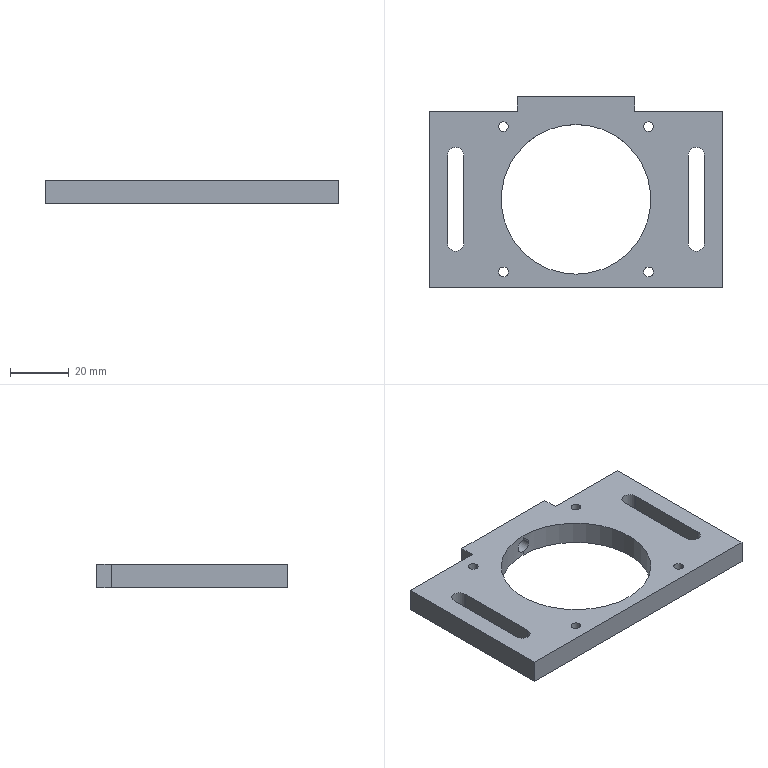Part | NX | features BREP 1 | 1 solid | 30 faces | box 100.003 x 65.003 x 8 mm | volume 29776 mm3 | cylinder 16 | plane 14 | commonest cylinder face diameters 3.3 x8 5.5 x4 5 x2 51 x2
STEP:
#1=CARTESIAN_POINT('',(-574.028,37.759,0.));
#2=VERTEX_POINT('',#1);
#3=CARTESIAN_POINT('',(-570.728,37.759,0.));
#4=VERTEX_POINT('',#3);
#5=CARTESIAN_POINT('',(-572.378,37.759,0.));
#6=DIRECTION('',(0.,0.,1.));
#7=DIRECTION('',(1.,0.,0.));
#8=AXIS2_PLACEMENT_3D('',#5,#6,#7);
#9=CIRCLE('',#8,1.65);
#10=EDGE_CURVE('',#2,#4,#9,.T.);
#11=ORIENTED_EDGE('',*,*,#10,.F.);
#12=CARTESIAN_POINT('',(-574.028,37.759,8.));
#13=VERTEX_POINT('',#12);
#14=CARTESIAN_POINT('',(-574.028,37.759,8.));
#15=DIRECTION('',(0.,0.,1.));
#16=VECTOR('',#15,1000.);
#17=LINE('',#14,#16);
#18=EDGE_CURVE('',#13,#2,#17,.F.);
#19=ORIENTED_EDGE('',*,*,#18,.F.);
#20=CARTESIAN_POINT('',(-570.728,37.759,8.));
#21=VERTEX_POINT('',#20);
#22=CARTESIAN_POINT('',(-572.378,37.759,8.));
#23=DIRECTION('',(0.,0.,1.));
#24=DIRECTION('',(1.,0.,0.));
#25=AXIS2_PLACEMENT_3D('',#22,#23,#24);
#26=CIRCLE('',#25,1.65);
#27=EDGE_CURVE('',#13,#21,#26,.T.);
#28=ORIENTED_EDGE('',*,*,#27,.T.);
#29=CARTESIAN_POINT('',(-570.728,37.759,8.));
#30=DIRECTION('',(0.,0.,1.));
#31=VECTOR('',#30,1000.);
#32=LINE('',#29,#31);
#33=EDGE_CURVE('',#21,#4,#32,.F.);
#34=ORIENTED_EDGE('',*,*,#33,.T.);
#35=EDGE_LOOP('',(#11,#19,#28,#34));
#36=FACE_BOUND('',#35,.T.);
#37=CARTESIAN_POINT('',(-572.378,37.759,8.));
#38=DIRECTION('',(0.,0.,1.));
#39=DIRECTION('',(1.,0.,0.));
#40=AXIS2_PLACEMENT_3D('',#37,#38,#39);
#41=CYLINDRICAL_SURFACE('',#40,1.65);
#42=ADVANCED_FACE('',(#36),#41,.F.);
#43=CARTESIAN_POINT('',(-524.531,37.761,0.));
#44=VERTEX_POINT('',#43);
#45=CARTESIAN_POINT('',(-521.231,37.761,0.));
#46=VERTEX_POINT('',#45);
#47=CARTESIAN_POINT('',(-522.881,37.761,0.));
#48=DIRECTION('',(0.,0.,1.));
#49=DIRECTION('',(1.,0.,0.));
#50=AXIS2_PLACEMENT_3D('',#47,#48,#49);
#51=CIRCLE('',#50,1.65);
#52=EDGE_CURVE('',#44,#46,#51,.T.);
#53=ORIENTED_EDGE('',*,*,#52,.F.);
#54=CARTESIAN_POINT('',(-524.531,37.761,8.));
#55=VERTEX_POINT('',#54);
#56=CARTESIAN_POINT('',(-524.531,37.761,8.));
#57=DIRECTION('',(0.,0.,1.));
#58=VECTOR('',#57,1000.);
#59=LINE('',#56,#58);
#60=EDGE_CURVE('',#55,#44,#59,.F.);
#61=ORIENTED_EDGE('',*,*,#60,.F.);
#62=CARTESIAN_POINT('',(-521.231,37.761,8.));
#63=VERTEX_POINT('',#62);
#64=CARTESIAN_POINT('',(-522.881,37.761,8.));
#65=DIRECTION('',(0.,0.,1.));
#66=DIRECTION('',(1.,0.,0.));
#67=AXIS2_PLACEMENT_3D('',#64,#65,#66);
#68=CIRCLE('',#67,1.65);
#69=EDGE_CURVE('',#55,#63,#68,.T.);
#70=ORIENTED_EDGE('',*,*,#69,.T.);
#71=CARTESIAN_POINT('',(-521.231,37.761,8.));
#72=DIRECTION('',(0.,0.,1.));
#73=VECTOR('',#72,1000.);
#74=LINE('',#71,#73);
#75=EDGE_CURVE('',#63,#46,#74,.F.);
#76=ORIENTED_EDGE('',*,*,#75,.T.);
#77=EDGE_LOOP('',(#53,#61,#70,#76));
#78=FACE_BOUND('',#77,.T.);
#79=CARTESIAN_POINT('',(-522.881,37.761,8.));
#80=DIRECTION('',(0.,0.,1.));
#81=DIRECTION('',(1.,0.,0.));
#82=AXIS2_PLACEMENT_3D('',#79,#80,#81);
#83=CYLINDRICAL_SURFACE('',#82,1.65);
#84=ADVANCED_FACE('',(#78),#83,.F.);
#85=CARTESIAN_POINT('',(-524.529,-11.736,0.));
#86=VERTEX_POINT('',#85);
#87=CARTESIAN_POINT('',(-521.229,-11.736,0.));
#88=VERTEX_POINT('',#87);
#89=CARTESIAN_POINT('',(-522.879,-11.736,0.));
#90=DIRECTION('',(0.,0.,1.));
#91=DIRECTION('',(1.,0.,0.));
#92=AXIS2_PLACEMENT_3D('',#89,#90,#91);
#93=CIRCLE('',#92,1.65);
#94=EDGE_CURVE('',#86,#88,#93,.T.);
#95=ORIENTED_EDGE('',*,*,#94,.F.);
#96=CARTESIAN_POINT('',(-524.529,-11.736,8.));
#97=VERTEX_POINT('',#96);
#98=CARTESIAN_POINT('',(-524.529,-11.736,8.));
#99=DIRECTION('',(0.,0.,1.));
#100=VECTOR('',#99,1000.);
#101=LINE('',#98,#100);
#102=EDGE_CURVE('',#97,#86,#101,.F.);
#103=ORIENTED_EDGE('',*,*,#102,.F.);
#104=CARTESIAN_POINT('',(-521.229,-11.736,8.));
#105=VERTEX_POINT('',#104);
#106=CARTESIAN_POINT('',(-522.879,-11.736,8.));
#107=DIRECTION('',(0.,0.,1.));
#108=DIRECTION('',(1.,0.,0.));
#109=AXIS2_PLACEMENT_3D('',#106,#107,#108);
#110=CIRCLE('',#109,1.65);
#111=EDGE_CURVE('',#97,#105,#110,.T.);
#112=ORIENTED_EDGE('',*,*,#111,.T.);
#113=CARTESIAN_POINT('',(-521.229,-11.736,8.));
#114=DIRECTION('',(0.,0.,1.));
#115=VECTOR('',#114,1000.);
#116=LINE('',#113,#115);
#117=EDGE_CURVE('',#105,#88,#116,.F.);
#118=ORIENTED_EDGE('',*,*,#117,.T.);
#119=EDGE_LOOP('',(#95,#103,#112,#118));
#120=FACE_BOUND('',#119,.T.);
#121=CARTESIAN_POINT('',(-522.879,-11.736,8.));
#122=DIRECTION('',(0.,0.,1.));
#123=DIRECTION('',(1.,0.,0.));
#124=AXIS2_PLACEMENT_3D('',#121,#122,#123);
#125=CYLINDRICAL_SURFACE('',#124,1.65);
#126=ADVANCED_FACE('',(#120),#125,.F.);
#127=CARTESIAN_POINT('',(-574.026,-11.739,0.));
#128=VERTEX_POINT('',#127);
#129=CARTESIAN_POINT('',(-570.726,-11.739,0.));
#130=VERTEX_POINT('',#129);
#131=CARTESIAN_POINT('',(-572.376,-11.739,0.));
#132=DIRECTION('',(0.,0.,1.));
#133=DIRECTION('',(1.,0.,0.));
#134=AXIS2_PLACEMENT_3D('',#131,#132,#133);
#135=CIRCLE('',#134,1.65);
#136=EDGE_CURVE('',#128,#130,#135,.T.);
#137=ORIENTED_EDGE('',*,*,#136,.F.);
#138=CARTESIAN_POINT('',(-574.026,-11.739,8.));
#139=VERTEX_POINT('',#138);
#140=CARTESIAN_POINT('',(-574.026,-11.739,8.));
#141=DIRECTION('',(0.,0.,1.));
#142=VECTOR('',#141,1000.);
#143=LINE('',#140,#142);
#144=EDGE_CURVE('',#139,#128,#143,.F.);
#145=ORIENTED_EDGE('',*,*,#144,.F.);
#146=CARTESIAN_POINT('',(-570.726,-11.739,8.));
#147=VERTEX_POINT('',#146);
#148=CARTESIAN_POINT('',(-572.376,-11.739,8.));
#149=DIRECTION('',(0.,0.,1.));
#150=DIRECTION('',(1.,0.,0.));
#151=AXIS2_PLACEMENT_3D('',#148,#149,#150);
#152=CIRCLE('',#151,1.65);
#153=EDGE_CURVE('',#139,#147,#152,.T.);
#154=ORIENTED_EDGE('',*,*,#153,.T.);
#155=CARTESIAN_POINT('',(-570.726,-11.739,8.));
#156=DIRECTION('',(0.,0.,1.));
#157=VECTOR('',#156,1000.);
#158=LINE('',#155,#157);
#159=EDGE_CURVE('',#147,#130,#158,.F.);
#160=ORIENTED_EDGE('',*,*,#159,.T.);
#161=EDGE_LOOP('',(#137,#145,#154,#160));
#162=FACE_BOUND('',#161,.T.);
#163=CARTESIAN_POINT('',(-572.376,-11.739,8.));
#164=DIRECTION('',(0.,0.,1.));
#165=DIRECTION('',(1.,0.,0.));
#166=AXIS2_PLACEMENT_3D('',#163,#164,#165);
#167=CYLINDRICAL_SURFACE('',#166,1.65);
#168=ADVANCED_FACE('',(#162),#167,.F.);
#169=CARTESIAN_POINT('',(-545.13,38.389,4.));
#170=VERTEX_POINT('',#169);
#171=CARTESIAN_POINT('',(-547.628,38.511,1.5));
#172=VERTEX_POINT('',#171);
#173=CARTESIAN_POINT('',(-547.628,38.511,1.5));
#174=CARTESIAN_POINT('',(-547.474,38.511,1.5));
#175=CARTESIAN_POINT('',(-547.166,38.509,1.523));
#176=CARTESIAN_POINT('',(-546.63,38.493,1.695));
#177=CARTESIAN_POINT('',(-546.34,38.479,1.843));
#178=CARTESIAN_POINT('',(-545.839,38.45,2.211));
#179=CARTESIAN_POINT('',(-545.471,38.421,2.714));
#180=CARTESIAN_POINT('',(-545.324,38.407,3.002));
#181=CARTESIAN_POINT('',(-545.152,38.391,3.538));
#182=CARTESIAN_POINT('',(-545.13,38.389,3.845));
#183=CARTESIAN_POINT('',(-545.13,38.389,4.));
#184=B_SPLINE_CURVE_WITH_KNOTS('',3,(#173,#174,#175,#176,#177,#178,#179,#180,#181,#182,#183),.UNSPECIFIED.,.F.,.F.,(4,1,1,1,1,1,1,1,4),(0.,0.125,0.25,0.375,0.5,0.625,0.75,0.875,1.),.UNSPECIFIED.);
#185=EDGE_CURVE('',#170,#172,#184,.F.);
#186=ORIENTED_EDGE('',*,*,#185,.F.);
#187=CARTESIAN_POINT('',(-545.13,48.011,4.));
#188=VERTEX_POINT('',#187);
#189=CARTESIAN_POINT('',(-545.13,48.011,4.));
#190=DIRECTION('',(-0.0000463,1.,0.));
#191=VECTOR('',#190,1000.);
#192=LINE('',#189,#191);
#193=EDGE_CURVE('',#170,#188,#192,.T.);
#194=ORIENTED_EDGE('',*,*,#193,.T.);
#195=CARTESIAN_POINT('',(-550.13,48.011,4.));
#196=VERTEX_POINT('',#195);
#197=CARTESIAN_POINT('',(-547.63,48.011,4.));
#198=DIRECTION('',(-0.0000463,1.,0.));
#199=DIRECTION('',(-1.,-0.0000463,0.));
#200=AXIS2_PLACEMENT_3D('',#197,#198,#199);
#201=CIRCLE('',#200,2.5);
#202=EDGE_CURVE('',#188,#196,#201,.T.);
#203=ORIENTED_EDGE('',*,*,#202,.T.);
#204=CARTESIAN_POINT('',(-550.13,38.388,4.));
#205=VERTEX_POINT('',#204);
#206=CARTESIAN_POINT('',(-550.13,48.011,4.));
#207=DIRECTION('',(-0.0000463,1.,0.));
#208=VECTOR('',#207,1000.);
#209=LINE('',#206,#208);
#210=EDGE_CURVE('',#205,#196,#209,.T.);
#211=ORIENTED_EDGE('',*,*,#210,.F.);
#212=CARTESIAN_POINT('',(-550.13,38.388,4.));
#213=CARTESIAN_POINT('',(-550.13,38.388,3.845));
#214=CARTESIAN_POINT('',(-550.107,38.391,3.537));
#215=CARTESIAN_POINT('',(-549.934,38.407,2.999));
#216=CARTESIAN_POINT('',(-549.787,38.42,2.712));
#217=CARTESIAN_POINT('',(-549.418,38.45,2.208));
#218=CARTESIAN_POINT('',(-548.918,38.479,1.843));
#219=CARTESIAN_POINT('',(-548.627,38.493,1.694));
#220=CARTESIAN_POINT('',(-548.091,38.509,1.522));
#221=CARTESIAN_POINT('',(-547.783,38.511,1.5));
#222=CARTESIAN_POINT('',(-547.628,38.511,1.5));
#223=B_SPLINE_CURVE_WITH_KNOTS('',3,(#212,#213,#214,#215,#216,#217,#218,#219,#220,#221,#222),.UNSPECIFIED.,.F.,.F.,(4,1,1,1,1,1,1,1,4),(0.,0.125,0.25,0.375,0.5,0.625,0.75,0.875,1.),.UNSPECIFIED.);
#224=EDGE_CURVE('',#172,#205,#223,.F.);
#225=ORIENTED_EDGE('',*,*,#224,.F.);
#226=EDGE_LOOP('',(#186,#194,#203,#211,#225));
#227=FACE_BOUND('',#226,.T.);
#228=CARTESIAN_POINT('',(-547.63,48.011,4.));
#229=DIRECTION('',(-0.0000463,1.,0.));
#230=DIRECTION('',(-1.,-0.0000463,0.));
#231=AXIS2_PLACEMENT_3D('',#228,#229,#230);
#232=CYLINDRICAL_SURFACE('',#231,2.5);
#233=ADVANCED_FACE('',(#227),#232,.F.);
#234=CARTESIAN_POINT('',(-547.628,38.511,0.));
#235=VERTEX_POINT('',#234);
#236=CARTESIAN_POINT('',(-547.628,-12.489,0.));
#237=VERTEX_POINT('',#236);
#238=CARTESIAN_POINT('',(-547.628,13.011,0.));
#239=DIRECTION('',(0.,0.,1.));
#240=DIRECTION('',(0.,-1.,0.));
#241=AXIS2_PLACEMENT_3D('',#238,#239,#240);
#242=CIRCLE('',#241,25.5);
#243=EDGE_CURVE('',#235,#237,#242,.T.);
#244=ORIENTED_EDGE('',*,*,#243,.F.);
#245=CARTESIAN_POINT('',(-547.628,38.511,0.));
#246=DIRECTION('',(0.,0.,1.));
#247=VECTOR('',#246,1000.);
#248=LINE('',#245,#247);
#249=EDGE_CURVE('',#172,#235,#248,.F.);
#250=ORIENTED_EDGE('',*,*,#249,.F.);
#251=ORIENTED_EDGE('',*,*,#224,.T.);
#252=CARTESIAN_POINT('',(-547.628,38.511,6.5));
#253=VERTEX_POINT('',#252);
#254=CARTESIAN_POINT('',(-550.13,38.388,4.));
#255=CARTESIAN_POINT('',(-550.13,38.388,4.657));
#256=CARTESIAN_POINT('',(-549.585,38.45,5.959));
#257=CARTESIAN_POINT('',(-548.285,38.511,6.5));
#258=CARTESIAN_POINT('',(-547.628,38.511,6.5));
#259=B_SPLINE_CURVE_WITH_KNOTS('',3,(#254,#255,#256,#257,#258),.UNSPECIFIED.,.F.,.F.,(4,1,4),(0.,0.5,1.),.UNSPECIFIED.);
#260=EDGE_CURVE('',#205,#253,#259,.T.);
#261=ORIENTED_EDGE('',*,*,#260,.T.);
#262=CARTESIAN_POINT('',(-547.628,38.511,8.));
#263=VERTEX_POINT('',#262);
#264=CARTESIAN_POINT('',(-547.628,38.511,0.));
#265=DIRECTION('',(0.,0.,1.));
#266=VECTOR('',#265,1000.);
#267=LINE('',#264,#266);
#268=EDGE_CURVE('',#253,#263,#267,.T.);
#269=ORIENTED_EDGE('',*,*,#268,.T.);
#270=CARTESIAN_POINT('',(-547.628,-12.489,8.));
#271=VERTEX_POINT('',#270);
#272=CARTESIAN_POINT('',(-547.628,13.011,8.));
#273=DIRECTION('',(0.,0.,1.));
#274=DIRECTION('',(0.,-1.,0.));
#275=AXIS2_PLACEMENT_3D('',#272,#273,#274);
#276=CIRCLE('',#275,25.5);
#277=EDGE_CURVE('',#263,#271,#276,.T.);
#278=ORIENTED_EDGE('',*,*,#277,.T.);
#279=CARTESIAN_POINT('',(-547.628,-12.489,0.));
#280=DIRECTION('',(0.,0.,1.));
#281=VECTOR('',#280,1000.);
#282=LINE('',#279,#281);
#283=EDGE_CURVE('',#271,#237,#282,.F.);
#284=ORIENTED_EDGE('',*,*,#283,.T.);
#285=EDGE_LOOP('',(#244,#250,#251,#261,#269,#278,#284));
#286=FACE_BOUND('',#285,.T.);
#287=CARTESIAN_POINT('',(-547.628,13.011,0.));
#288=DIRECTION('',(0.,0.,1.));
#289=DIRECTION('',(0.,-1.,0.));
#290=AXIS2_PLACEMENT_3D('',#287,#288,#289);
#291=CYLINDRICAL_SURFACE('',#290,25.5);
#292=ADVANCED_FACE('',(#286),#291,.F.);
#293=CARTESIAN_POINT('',(-497.627,-16.986,0.));
#294=VERTEX_POINT('',#293);
#295=CARTESIAN_POINT('',(-497.63,43.014,0.));
#296=VERTEX_POINT('',#295);
#297=CARTESIAN_POINT('',(-497.627,-16.986,0.));
#298=DIRECTION('',(-0.0000463,1.,0.));
#299=VECTOR('',#298,1000.);
#300=LINE('',#297,#299);
#301=EDGE_CURVE('',#294,#296,#300,.T.);
#302=ORIENTED_EDGE('',*,*,#301,.T.);
#303=CARTESIAN_POINT('',(-497.63,43.014,8.));
#304=VERTEX_POINT('',#303);
#305=CARTESIAN_POINT('',(-497.63,43.014,8.));
#306=DIRECTION('',(0.,0.,-1.));
#307=VECTOR('',#306,1000.);
#308=LINE('',#305,#307);
#309=EDGE_CURVE('',#304,#296,#308,.T.);
#310=ORIENTED_EDGE('',*,*,#309,.F.);
#311=CARTESIAN_POINT('',(-497.627,-16.986,8.));
#312=VERTEX_POINT('',#311);
#313=CARTESIAN_POINT('',(-497.627,-16.986,8.));
#314=DIRECTION('',(-0.0000463,1.,0.));
#315=VECTOR('',#314,1000.);
#316=LINE('',#313,#315);
#317=EDGE_CURVE('',#312,#304,#316,.T.);
#318=ORIENTED_EDGE('',*,*,#317,.F.);
#319=CARTESIAN_POINT('',(-497.627,-16.986,8.));
#320=DIRECTION('',(0.,0.,-1.));
#321=VECTOR('',#320,1000.);
#322=LINE('',#319,#321);
#323=EDGE_CURVE('',#312,#294,#322,.T.);
#324=ORIENTED_EDGE('',*,*,#323,.T.);
#325=EDGE_LOOP('',(#302,#310,#318,#324));
#326=FACE_BOUND('',#325,.T.);
#327=CARTESIAN_POINT('',(-497.627,-16.986,8.));
#328=DIRECTION('',(-1.,-0.0000463,0.));
#329=DIRECTION('',(-0.0000463,1.,0.));
#330=AXIS2_PLACEMENT_3D('',#327,#328,#329);
#331=PLANE('',#330);
#332=ADVANCED_FACE('',(#326),#331,.F.);
#333=CARTESIAN_POINT('',(-527.63,43.012,0.));
#334=VERTEX_POINT('',#333);
#335=CARTESIAN_POINT('',(-497.63,43.014,0.));
#336=DIRECTION('',(-1.,-0.0000463,0.));
#337=VECTOR('',#336,1000.);
#338=LINE('',#335,#337);
#339=EDGE_CURVE('',#296,#334,#338,.T.);
#340=ORIENTED_EDGE('',*,*,#339,.T.);
#341=CARTESIAN_POINT('',(-527.63,43.012,8.));
#342=VERTEX_POINT('',#341);
#343=CARTESIAN_POINT('',(-527.63,43.012,8.));
#344=DIRECTION('',(0.,0.,-1.));
#345=VECTOR('',#344,1000.);
#346=LINE('',#343,#345);
#347=EDGE_CURVE('',#342,#334,#346,.T.);
#348=ORIENTED_EDGE('',*,*,#347,.F.);
#349=CARTESIAN_POINT('',(-497.63,43.014,8.));
#350=DIRECTION('',(-1.,-0.0000463,0.));
#351=VECTOR('',#350,1000.);
#352=LINE('',#349,#351);
#353=EDGE_CURVE('',#304,#342,#352,.T.);
#354=ORIENTED_EDGE('',*,*,#353,.F.);
#355=ORIENTED_EDGE('',*,*,#309,.T.);
#356=EDGE_LOOP('',(#340,#348,#354,#355));
#357=FACE_BOUND('',#356,.T.);
#358=CARTESIAN_POINT('',(-497.63,43.014,8.));
#359=DIRECTION('',(0.0000463,-1.,0.));
#360=DIRECTION('',(0.,0.,-1.));
#361=AXIS2_PLACEMENT_3D('',#358,#359,#360);
#362=PLANE('',#361);
#363=ADVANCED_FACE('',(#357),#362,.F.);
#364=CARTESIAN_POINT('',(-527.63,48.012,0.));
#365=VERTEX_POINT('',#364);
#366=CARTESIAN_POINT('',(-527.63,48.012,0.));
#367=DIRECTION('',(-0.0000463,1.,0.));
#368=VECTOR('',#367,1000.);
#369=LINE('',#366,#368);
#370=EDGE_CURVE('',#334,#365,#369,.T.);
#371=ORIENTED_EDGE('',*,*,#370,.T.);
#372=CARTESIAN_POINT('',(-527.63,48.012,8.));
#373=VERTEX_POINT('',#372);
#374=CARTESIAN_POINT('',(-527.63,48.012,8.));
#375=DIRECTION('',(0.,0.,-1.));
#376=VECTOR('',#375,1000.);
#377=LINE('',#374,#376);
#378=EDGE_CURVE('',#373,#365,#377,.T.);
#379=ORIENTED_EDGE('',*,*,#378,.F.);
#380=CARTESIAN_POINT('',(-527.63,48.012,8.));
#381=DIRECTION('',(-0.0000463,1.,0.));
#382=VECTOR('',#381,1000.);
#383=LINE('',#380,#382);
#384=EDGE_CURVE('',#342,#373,#383,.T.);
#385=ORIENTED_EDGE('',*,*,#384,.F.);
#386=ORIENTED_EDGE('',*,*,#347,.T.);
#387=EDGE_LOOP('',(#371,#379,#385,#386));
#388=FACE_BOUND('',#387,.T.);
#389=CARTESIAN_POINT('',(-527.63,48.012,8.));
#390=DIRECTION('',(-1.,-0.0000463,0.));
#391=DIRECTION('',(-0.0000463,1.,0.));
#392=AXIS2_PLACEMENT_3D('',#389,#390,#391);
#393=PLANE('',#392);
#394=ADVANCED_FACE('',(#388),#393,.F.);
#395=CARTESIAN_POINT('',(-567.63,48.01,0.));
#396=VERTEX_POINT('',#395);
#397=CARTESIAN_POINT('',(-527.63,48.012,0.));
#398=DIRECTION('',(-1.,-0.0000463,0.));
#399=VECTOR('',#398,1000.);
#400=LINE('',#397,#399);
#401=EDGE_CURVE('',#365,#396,#400,.T.);
#402=ORIENTED_EDGE('',*,*,#401,.T.);
#403=CARTESIAN_POINT('',(-567.63,48.01,8.));
#404=VERTEX_POINT('',#403);
#405=CARTESIAN_POINT('',(-567.63,48.01,8.));
#406=DIRECTION('',(0.,0.,-1.));
#407=VECTOR('',#406,1000.);
#408=LINE('',#405,#407);
#409=EDGE_CURVE('',#404,#396,#408,.T.);
#410=ORIENTED_EDGE('',*,*,#409,.F.);
#411=CARTESIAN_POINT('',(-527.63,48.012,8.));
#412=DIRECTION('',(-1.,-0.0000463,0.));
#413=VECTOR('',#412,1000.);
#414=LINE('',#411,#413);
#415=EDGE_CURVE('',#373,#404,#414,.T.);
#416=ORIENTED_EDGE('',*,*,#415,.F.);
#417=ORIENTED_EDGE('',*,*,#378,.T.);
#418=EDGE_LOOP('',(#402,#410,#416,#417));
#419=FACE_BOUND('',#418,.T.);
#420=CARTESIAN_POINT('',(-547.63,48.011,4.));
#421=DIRECTION('',(-0.0000463,1.,0.));
#422=DIRECTION('',(-1.,-0.0000463,0.));
#423=AXIS2_PLACEMENT_3D('',#420,#421,#422);
#424=CIRCLE('',#423,2.5);
#425=EDGE_CURVE('',#196,#188,#424,.T.);
#426=ORIENTED_EDGE('',*,*,#425,.F.);
#427=ORIENTED_EDGE('',*,*,#202,.F.);
#428=EDGE_LOOP('',(#426,#427));
#429=FACE_BOUND('',#428,.T.);
#430=CARTESIAN_POINT('',(-527.63,48.012,8.));
#431=DIRECTION('',(0.0000463,-1.,0.));
#432=DIRECTION('',(0.,0.,-1.));
#433=AXIS2_PLACEMENT_3D('',#430,#431,#432);
#434=PLANE('',#433);
#435=ADVANCED_FACE('',(#419,#429),#434,.F.);
#436=CARTESIAN_POINT('',(-567.63,43.01,0.));
#437=VERTEX_POINT('',#436);
#438=CARTESIAN_POINT('',(-567.63,48.01,0.));
#439=DIRECTION('',(0.0000463,-1.,0.));
#440=VECTOR('',#439,1000.);
#441=LINE('',#438,#440);
#442=EDGE_CURVE('',#396,#437,#441,.T.);
#443=ORIENTED_EDGE('',*,*,#442,.T.);
#444=CARTESIAN_POINT('',(-567.63,43.01,8.));
#445=VERTEX_POINT('',#444);
#446=CARTESIAN_POINT('',(-567.63,43.01,8.));
#447=DIRECTION('',(0.,0.,-1.));
#448=VECTOR('',#447,1000.);
#449=LINE('',#446,#448);
#450=EDGE_CURVE('',#445,#437,#449,.T.);
#451=ORIENTED_EDGE('',*,*,#450,.F.);
#452=CARTESIAN_POINT('',(-567.63,48.01,8.));
#453=DIRECTION('',(0.0000463,-1.,0.));
#454=VECTOR('',#453,1000.);
#455=LINE('',#452,#454);
#456=EDGE_CURVE('',#404,#445,#455,.T.);
#457=ORIENTED_EDGE('',*,*,#456,.F.);
#458=ORIENTED_EDGE('',*,*,#409,.T.);
#459=EDGE_LOOP('',(#443,#451,#457,#458));
#460=FACE_BOUND('',#459,.T.);
#461=CARTESIAN_POINT('',(-567.63,48.01,8.));
#462=DIRECTION('',(1.,0.0000463,0.));
#463=DIRECTION('',(0.,0.,-1.));
#464=AXIS2_PLACEMENT_3D('',#461,#462,#463);
#465=PLANE('',#464);
#466=ADVANCED_FACE('',(#460),#465,.F.);
#467=CARTESIAN_POINT('',(-597.63,43.009,0.));
#468=VERTEX_POINT('',#467);
#469=CARTESIAN_POINT('',(-567.63,43.01,0.));
#470=DIRECTION('',(-1.,-0.0000463,0.));
#471=VECTOR('',#470,1000.);
#472=LINE('',#469,#471);
#473=EDGE_CURVE('',#437,#468,#472,.T.);
#474=ORIENTED_EDGE('',*,*,#473,.T.);
#475=CARTESIAN_POINT('',(-597.63,43.009,8.));
#476=VERTEX_POINT('',#475);
#477=CARTESIAN_POINT('',(-597.63,43.009,8.));
#478=DIRECTION('',(0.,0.,-1.));
#479=VECTOR('',#478,1000.);
#480=LINE('',#477,#479);
#481=EDGE_CURVE('',#476,#468,#480,.T.);
#482=ORIENTED_EDGE('',*,*,#481,.F.);
#483=CARTESIAN_POINT('',(-567.63,43.01,8.));
#484=DIRECTION('',(-1.,-0.0000463,0.));
#485=VECTOR('',#484,1000.);
#486=LINE('',#483,#485);
#487=EDGE_CURVE('',#445,#476,#486,.T.);
#488=ORIENTED_EDGE('',*,*,#487,.F.);
#489=ORIENTED_EDGE('',*,*,#450,.T.);
#490=EDGE_LOOP('',(#474,#482,#488,#489));
#491=FACE_BOUND('',#490,.T.);
#492=CARTESIAN_POINT('',(-567.63,43.01,8.));
#493=DIRECTION('',(0.0000463,-1.,0.));
#494=DIRECTION('',(0.,0.,-1.));
#495=AXIS2_PLACEMENT_3D('',#492,#493,#494);
#496=PLANE('',#495);
#497=ADVANCED_FACE('',(#491),#496,.F.);
#498=CARTESIAN_POINT('',(-597.627,-16.991,0.));
#499=VERTEX_POINT('',#498);
#500=CARTESIAN_POINT('',(-597.627,-16.991,0.));
#501=DIRECTION('',(0.0000463,-1.,0.));
#502=VECTOR('',#501,1000.);
#503=LINE('',#500,#502);
#504=EDGE_CURVE('',#468,#499,#503,.T.);
#505=ORIENTED_EDGE('',*,*,#504,.T.);
#506=CARTESIAN_POINT('',(-597.627,-16.991,8.));
#507=VERTEX_POINT('',#506);
#508=CARTESIAN_POINT('',(-597.627,-16.991,8.));
#509=DIRECTION('',(0.,0.,-1.));
#510=VECTOR('',#509,1000.);
#511=LINE('',#508,#510);
#512=EDGE_CURVE('',#507,#499,#511,.T.);
#513=ORIENTED_EDGE('',*,*,#512,.F.);
#514=CARTESIAN_POINT('',(-597.627,-16.991,8.));
#515=DIRECTION('',(0.0000463,-1.,0.));
#516=VECTOR('',#515,1000.);
#517=LINE('',#514,#516);
#518=EDGE_CURVE('',#476,#507,#517,.T.);
#519=ORIENTED_EDGE('',*,*,#518,.F.);
#520=ORIENTED_EDGE('',*,*,#481,.T.);
#521=EDGE_LOOP('',(#505,#513,#519,#520));
#522=FACE_BOUND('',#521,.T.);
#523=CARTESIAN_POINT('',(-597.627,-16.991,8.));
#524=DIRECTION('',(1.,0.0000463,0.));
#525=DIRECTION('',(0.,0.,-1.));
#526=AXIS2_PLACEMENT_3D('',#523,#524,#525);
#527=PLANE('',#526);
#528=ADVANCED_FACE('',(#522),#527,.F.);
#529=CARTESIAN_POINT('',(-497.627,-16.986,0.));
#530=DIRECTION('',(1.,0.0000463,0.));
#531=VECTOR('',#530,1000.);
#532=LINE('',#529,#531);
#533=EDGE_CURVE('',#499,#294,#532,.T.);
#534=ORIENTED_EDGE('',*,*,#533,.T.);
#535=ORIENTED_EDGE('',*,*,#323,.F.);
#536=CARTESIAN_POINT('',(-497.627,-16.986,8.));
#537=DIRECTION('',(1.,0.0000463,0.));
#538=VECTOR('',#537,1000.);
#539=LINE('',#536,#538);
#540=EDGE_CURVE('',#507,#312,#539,.T.);
#541=ORIENTED_EDGE('',*,*,#540,.F.);
#542=ORIENTED_EDGE('',*,*,#512,.T.);
#543=EDGE_LOOP('',(#534,#535,#541,#542));
#544=FACE_BOUND('',#543,.T.);
#545=CARTESIAN_POINT('',(-497.627,-16.986,8.));
#546=DIRECTION('',(-0.0000463,1.,0.));
#547=DIRECTION('',(0.,0.,1.));
#548=AXIS2_PLACEMENT_3D('',#545,#546,#547);
#549=PLANE('',#548);
#550=ADVANCED_FACE('',(#544),#549,.F.);
#551=ORIENTED_EDGE('',*,*,#317,.T.);
#552=ORIENTED_EDGE('',*,*,#353,.T.);
#553=ORIENTED_EDGE('',*,*,#384,.T.);
#554=ORIENTED_EDGE('',*,*,#415,.T.);
#555=ORIENTED_EDGE('',*,*,#456,.T.);
#556=ORIENTED_EDGE('',*,*,#487,.T.);
#557=ORIENTED_EDGE('',*,*,#518,.T.);
#558=ORIENTED_EDGE('',*,*,#540,.T.);
#559=EDGE_LOOP('',(#551,#552,#553,#554,#555,#556,#557,#558));
#560=FACE_BOUND('',#559,.T.);
#561=CARTESIAN_POINT('',(-572.378,37.759,8.));
#562=DIRECTION('',(0.,0.,1.));
#563=DIRECTION('',(1.,0.,0.));
#564=AXIS2_PLACEMENT_3D('',#561,#562,#563);
#565=CIRCLE('',#564,1.65);
#566=EDGE_CURVE('',#21,#13,#565,.T.);
#567=ORIENTED_EDGE('',*,*,#566,.F.);
#568=ORIENTED_EDGE('',*,*,#27,.F.);
#569=EDGE_LOOP('',(#567,#568));
#570=FACE_BOUND('',#569,.T.);
#571=CARTESIAN_POINT('',(-522.881,37.761,8.));
#572=DIRECTION('',(0.,0.,1.));
#573=DIRECTION('',(1.,0.,0.));
#574=AXIS2_PLACEMENT_3D('',#571,#572,#573);
#575=CIRCLE('',#574,1.65);
#576=EDGE_CURVE('',#63,#55,#575,.T.);
#577=ORIENTED_EDGE('',*,*,#576,.F.);
#578=ORIENTED_EDGE('',*,*,#69,.F.);
#579=EDGE_LOOP('',(#577,#578));
#580=FACE_BOUND('',#579,.T.);
#581=CARTESIAN_POINT('',(-522.879,-11.736,8.));
#582=DIRECTION('',(0.,0.,1.));
#583=DIRECTION('',(1.,0.,0.));
#584=AXIS2_PLACEMENT_3D('',#581,#582,#583);
#585=CIRCLE('',#584,1.65);
#586=EDGE_CURVE('',#105,#97,#585,.T.);
#587=ORIENTED_EDGE('',*,*,#586,.F.);
#588=ORIENTED_EDGE('',*,*,#111,.F.);
#589=EDGE_LOOP('',(#587,#588));
#590=FACE_BOUND('',#589,.T.);
#591=CARTESIAN_POINT('',(-572.376,-11.739,8.));
#592=DIRECTION('',(0.,0.,1.));
#593=DIRECTION('',(1.,0.,0.));
#594=AXIS2_PLACEMENT_3D('',#591,#592,#593);
#595=CIRCLE('',#594,1.65);
#596=EDGE_CURVE('',#147,#139,#595,.T.);
#597=ORIENTED_EDGE('',*,*,#596,.F.);
#598=ORIENTED_EDGE('',*,*,#153,.F.);
#599=EDGE_LOOP('',(#597,#598));
#600=FACE_BOUND('',#599,.T.);
#601=CARTESIAN_POINT('',(-585.875,28.014,8.));
#602=VERTEX_POINT('',#601);
#603=CARTESIAN_POINT('',(-591.375,28.014,8.));
#604=VERTEX_POINT('',#603);
#605=CARTESIAN_POINT('',(-588.625,28.014,8.));
#606=DIRECTION('',(0.,0.,1.));
#607=DIRECTION('',(-1.,0.,0.));
#608=AXIS2_PLACEMENT_3D('',#605,#606,#607);
#609=CIRCLE('',#608,2.75);
#610=EDGE_CURVE('',#602,#604,#609,.T.);
#611=ORIENTED_EDGE('',*,*,#610,.F.);
#612=CARTESIAN_POINT('',(-585.875,-1.986,8.));
#613=VERTEX_POINT('',#612);
#614=CARTESIAN_POINT('',(-585.875,28.014,8.));
#615=DIRECTION('',(0.,1.,0.));
#616=VECTOR('',#615,1000.);
#617=LINE('',#614,#616);
#618=EDGE_CURVE('',#613,#602,#617,.T.);
#619=ORIENTED_EDGE('',*,*,#618,.F.);
#620=CARTESIAN_POINT('',(-591.375,-1.986,8.));
#621=VERTEX_POINT('',#620);
#622=CARTESIAN_POINT('',(-588.625,-1.986,8.));
#623=DIRECTION('',(0.,0.,1.));
#624=DIRECTION('',(-1.,0.,0.));
#625=AXIS2_PLACEMENT_3D('',#622,#623,#624);
#626=CIRCLE('',#625,2.75);
#627=EDGE_CURVE('',#621,#613,#626,.T.);
#628=ORIENTED_EDGE('',*,*,#627,.F.);
#629=CARTESIAN_POINT('',(-591.375,28.014,8.));
#630=DIRECTION('',(0.,-1.,0.));
#631=VECTOR('',#630,1000.);
#632=LINE('',#629,#631);
#633=EDGE_CURVE('',#604,#621,#632,.T.);
#634=ORIENTED_EDGE('',*,*,#633,.F.);
#635=EDGE_LOOP('',(#611,#619,#628,#634));
#636=FACE_BOUND('',#635,.T.);
#637=CARTESIAN_POINT('',(-503.879,28.014,8.));
#638=VERTEX_POINT('',#637);
#639=CARTESIAN_POINT('',(-509.379,28.014,8.));
#640=VERTEX_POINT('',#639);
#641=CARTESIAN_POINT('',(-506.629,28.014,8.));
#642=DIRECTION('',(0.,0.,1.));
#643=DIRECTION('',(1.,0.,0.));
#644=AXIS2_PLACEMENT_3D('',#641,#642,#643);
#645=CIRCLE('',#644,2.75);
#646=EDGE_CURVE('',#638,#640,#645,.T.);
#647=ORIENTED_EDGE('',*,*,#646,.F.);
#648=CARTESIAN_POINT('',(-503.879,-1.986,8.));
#649=VERTEX_POINT('',#648);
#650=CARTESIAN_POINT('',(-503.879,28.014,8.));
#651=DIRECTION('',(0.,1.,0.));
#652=VECTOR('',#651,1000.);
#653=LINE('',#650,#652);
#654=EDGE_CURVE('',#649,#638,#653,.T.);
#655=ORIENTED_EDGE('',*,*,#654,.F.);
#656=CARTESIAN_POINT('',(-509.379,-1.986,8.));
#657=VERTEX_POINT('',#656);
#658=CARTESIAN_POINT('',(-506.629,-1.986,8.));
#659=DIRECTION('',(0.,0.,1.));
#660=DIRECTION('',(1.,0.,0.));
#661=AXIS2_PLACEMENT_3D('',#658,#659,#660);
#662=CIRCLE('',#661,2.75);
#663=EDGE_CURVE('',#657,#649,#662,.T.);
#664=ORIENTED_EDGE('',*,*,#663,.F.);
#665=CARTESIAN_POINT('',(-509.379,28.014,8.));
#666=DIRECTION('',(0.,-1.,0.));
#667=VECTOR('',#666,1000.);
#668=LINE('',#665,#667);
#669=EDGE_CURVE('',#640,#657,#668,.T.);
#670=ORIENTED_EDGE('',*,*,#669,.F.);
#671=EDGE_LOOP('',(#647,#655,#664,#670));
#672=FACE_BOUND('',#671,.T.);
#673=CARTESIAN_POINT('',(-547.628,13.011,8.));
#674=DIRECTION('',(0.,0.,1.));
#675=DIRECTION('',(0.,-1.,0.));
#676=AXIS2_PLACEMENT_3D('',#673,#674,#675);
#677=CIRCLE('',#676,25.5);
#678=EDGE_CURVE('',#271,#263,#677,.T.);
#679=ORIENTED_EDGE('',*,*,#678,.F.);
#680=ORIENTED_EDGE('',*,*,#277,.F.);
#681=EDGE_LOOP('',(#679,#680));
#682=FACE_BOUND('',#681,.T.);
#683=CARTESIAN_POINT('',(-497.63,43.014,8.));
#684=DIRECTION('',(0.,0.,1.));
#685=DIRECTION('',(1.,0.,0.));
#686=AXIS2_PLACEMENT_3D('',#683,#684,#685);
#687=PLANE('',#686);
#688=ADVANCED_FACE('',(#560,#570,#580,#590,#600,#636,#672,#682),#687,.T.);
#689=ORIENTED_EDGE('',*,*,#301,.F.);
#690=ORIENTED_EDGE('',*,*,#533,.F.);
#691=ORIENTED_EDGE('',*,*,#504,.F.);
#692=ORIENTED_EDGE('',*,*,#473,.F.);
#693=ORIENTED_EDGE('',*,*,#442,.F.);
#694=ORIENTED_EDGE('',*,*,#401,.F.);
#695=ORIENTED_EDGE('',*,*,#370,.F.);
#696=ORIENTED_EDGE('',*,*,#339,.F.);
#697=EDGE_LOOP('',(#689,#690,#691,#692,#693,#694,#695,#696));
#698=FACE_BOUND('',#697,.T.);
#699=CARTESIAN_POINT('',(-572.378,37.759,0.));
#700=DIRECTION('',(0.,0.,1.));
#701=DIRECTION('',(1.,0.,0.));
#702=AXIS2_PLACEMENT_3D('',#699,#700,#701);
#703=CIRCLE('',#702,1.65);
#704=EDGE_CURVE('',#4,#2,#703,.T.);
#705=ORIENTED_EDGE('',*,*,#704,.T.);
#706=ORIENTED_EDGE('',*,*,#10,.T.);
#707=EDGE_LOOP('',(#705,#706));
#708=FACE_BOUND('',#707,.T.);
#709=CARTESIAN_POINT('',(-522.881,37.761,0.));
#710=DIRECTION('',(0.,0.,1.));
#711=DIRECTION('',(1.,0.,0.));
#712=AXIS2_PLACEMENT_3D('',#709,#710,#711);
#713=CIRCLE('',#712,1.65);
#714=EDGE_CURVE('',#46,#44,#713,.T.);
#715=ORIENTED_EDGE('',*,*,#714,.T.);
#716=ORIENTED_EDGE('',*,*,#52,.T.);
#717=EDGE_LOOP('',(#715,#716));
#718=FACE_BOUND('',#717,.T.);
#719=CARTESIAN_POINT('',(-522.879,-11.736,0.));
#720=DIRECTION('',(0.,0.,1.));
#721=DIRECTION('',(1.,0.,0.));
#722=AXIS2_PLACEMENT_3D('',#719,#720,#721);
#723=CIRCLE('',#722,1.65);
#724=EDGE_CURVE('',#88,#86,#723,.T.);
#725=ORIENTED_EDGE('',*,*,#724,.T.);
#726=ORIENTED_EDGE('',*,*,#94,.T.);
#727=EDGE_LOOP('',(#725,#726));
#728=FACE_BOUND('',#727,.T.);
#729=CARTESIAN_POINT('',(-572.376,-11.739,0.));
#730=DIRECTION('',(0.,0.,1.));
#731=DIRECTION('',(1.,0.,0.));
#732=AXIS2_PLACEMENT_3D('',#729,#730,#731);
#733=CIRCLE('',#732,1.65);
#734=EDGE_CURVE('',#130,#128,#733,.T.);
#735=ORIENTED_EDGE('',*,*,#734,.T.);
#736=ORIENTED_EDGE('',*,*,#136,.T.);
#737=EDGE_LOOP('',(#735,#736));
#738=FACE_BOUND('',#737,.T.);
#739=CARTESIAN_POINT('',(-585.875,-1.986,0.));
#740=VERTEX_POINT('',#739);
#741=CARTESIAN_POINT('',(-585.875,28.014,0.));
#742=VERTEX_POINT('',#741);
#743=CARTESIAN_POINT('',(-585.875,28.014,0.));
#744=DIRECTION('',(0.,1.,0.));
#745=VECTOR('',#744,1000.);
#746=LINE('',#743,#745);
#747=EDGE_CURVE('',#740,#742,#746,.T.);
#748=ORIENTED_EDGE('',*,*,#747,.T.);
#749=CARTESIAN_POINT('',(-591.375,28.014,0.));
#750=VERTEX_POINT('',#749);
#751=CARTESIAN_POINT('',(-588.625,28.014,0.));
#752=DIRECTION('',(0.,0.,1.));
#753=DIRECTION('',(-1.,0.,0.));
#754=AXIS2_PLACEMENT_3D('',#751,#752,#753);
#755=CIRCLE('',#754,2.75);
#756=EDGE_CURVE('',#742,#750,#755,.T.);
#757=ORIENTED_EDGE('',*,*,#756,.T.);
#758=CARTESIAN_POINT('',(-591.375,-1.986,0.));
#759=VERTEX_POINT('',#758);
#760=CARTESIAN_POINT('',(-591.375,28.014,0.));
#761=DIRECTION('',(0.,-1.,0.));
#762=VECTOR('',#761,1000.);
#763=LINE('',#760,#762);
#764=EDGE_CURVE('',#750,#759,#763,.T.);
#765=ORIENTED_EDGE('',*,*,#764,.T.);
#766=CARTESIAN_POINT('',(-588.625,-1.986,0.));
#767=DIRECTION('',(0.,0.,1.));
#768=DIRECTION('',(-1.,0.,0.));
#769=AXIS2_PLACEMENT_3D('',#766,#767,#768);
#770=CIRCLE('',#769,2.75);
#771=EDGE_CURVE('',#759,#740,#770,.T.);
#772=ORIENTED_EDGE('',*,*,#771,.T.);
#773=EDGE_LOOP('',(#748,#757,#765,#772));
#774=FACE_BOUND('',#773,.T.);
#775=CARTESIAN_POINT('',(-503.879,-1.986,0.));
#776=VERTEX_POINT('',#775);
#777=CARTESIAN_POINT('',(-503.879,28.014,0.));
#778=VERTEX_POINT('',#777);
#779=CARTESIAN_POINT('',(-503.879,28.014,0.));
#780=DIRECTION('',(0.,1.,0.));
#781=VECTOR('',#780,1000.);
#782=LINE('',#779,#781);
#783=EDGE_CURVE('',#776,#778,#782,.T.);
#784=ORIENTED_EDGE('',*,*,#783,.T.);
#785=CARTESIAN_POINT('',(-509.379,28.014,0.));
#786=VERTEX_POINT('',#785);
#787=CARTESIAN_POINT('',(-506.629,28.014,0.));
#788=DIRECTION('',(0.,0.,1.));
#789=DIRECTION('',(1.,0.,0.));
#790=AXIS2_PLACEMENT_3D('',#787,#788,#789);
#791=CIRCLE('',#790,2.75);
#792=EDGE_CURVE('',#778,#786,#791,.T.);
#793=ORIENTED_EDGE('',*,*,#792,.T.);
#794=CARTESIAN_POINT('',(-509.379,-1.986,0.));
#795=VERTEX_POINT('',#794);
#796=CARTESIAN_POINT('',(-509.379,28.014,0.));
#797=DIRECTION('',(0.,-1.,0.));
#798=VECTOR('',#797,1000.);
#799=LINE('',#796,#798);
#800=EDGE_CURVE('',#786,#795,#799,.T.);
#801=ORIENTED_EDGE('',*,*,#800,.T.);
#802=CARTESIAN_POINT('',(-506.629,-1.986,0.));
#803=DIRECTION('',(0.,0.,1.));
#804=DIRECTION('',(1.,0.,0.));
#805=AXIS2_PLACEMENT_3D('',#802,#803,#804);
#806=CIRCLE('',#805,2.75);
#807=EDGE_CURVE('',#795,#776,#806,.T.);
#808=ORIENTED_EDGE('',*,*,#807,.T.);
#809=EDGE_LOOP('',(#784,#793,#801,#808));
#810=FACE_BOUND('',#809,.T.);
#811=CARTESIAN_POINT('',(-547.628,13.011,0.));
#812=DIRECTION('',(0.,0.,1.));
#813=DIRECTION('',(0.,-1.,0.));
#814=AXIS2_PLACEMENT_3D('',#811,#812,#813);
#815=CIRCLE('',#814,25.5);
#816=EDGE_CURVE('',#237,#235,#815,.T.);
#817=ORIENTED_EDGE('',*,*,#816,.T.);
#818=ORIENTED_EDGE('',*,*,#243,.T.);
#819=EDGE_LOOP('',(#817,#818));
#820=FACE_BOUND('',#819,.T.);
#821=CARTESIAN_POINT('',(-497.63,43.014,0.));
#822=DIRECTION('',(0.,0.,1.));
#823=DIRECTION('',(1.,0.,0.));
#824=AXIS2_PLACEMENT_3D('',#821,#822,#823);
#825=PLANE('',#824);
#826=ADVANCED_FACE('',(#698,#708,#718,#728,#738,#774,#810,#820),#825,.F.);
#827=ORIENTED_EDGE('',*,*,#249,.T.);
#828=ORIENTED_EDGE('',*,*,#816,.F.);
#829=ORIENTED_EDGE('',*,*,#283,.F.);
#830=ORIENTED_EDGE('',*,*,#678,.T.);
#831=ORIENTED_EDGE('',*,*,#268,.F.);
#832=CARTESIAN_POINT('',(-547.628,38.511,6.5));
#833=CARTESIAN_POINT('',(-546.97,38.511,6.5));
#834=CARTESIAN_POINT('',(-545.673,38.45,5.956));
#835=CARTESIAN_POINT('',(-545.13,38.389,4.657));
#836=CARTESIAN_POINT('',(-545.13,38.389,4.));
#837=B_SPLINE_CURVE_WITH_KNOTS('',3,(#832,#833,#834,#835,#836),.UNSPECIFIED.,.F.,.F.,(4,1,4),(0.,0.5,1.),.UNSPECIFIED.);
#838=EDGE_CURVE('',#253,#170,#837,.T.);
#839=ORIENTED_EDGE('',*,*,#838,.T.);
#840=ORIENTED_EDGE('',*,*,#185,.T.);
#841=EDGE_LOOP('',(#827,#828,#829,#830,#831,#839,#840));
#842=FACE_BOUND('',#841,.T.);
#843=CARTESIAN_POINT('',(-547.628,13.011,0.));
#844=DIRECTION('',(0.,0.,1.));
#845=DIRECTION('',(0.,-1.,0.));
#846=AXIS2_PLACEMENT_3D('',#843,#844,#845);
#847=CYLINDRICAL_SURFACE('',#846,25.5);
#848=ADVANCED_FACE('',(#842),#847,.F.);
#849=ORIENTED_EDGE('',*,*,#646,.T.);
#850=CARTESIAN_POINT('',(-509.379,28.014,0.));
#851=DIRECTION('',(0.,0.,1.));
#852=VECTOR('',#851,1000.);
#853=LINE('',#850,#852);
#854=EDGE_CURVE('',#786,#640,#853,.T.);
#855=ORIENTED_EDGE('',*,*,#854,.F.);
#856=ORIENTED_EDGE('',*,*,#792,.F.);
#857=CARTESIAN_POINT('',(-503.879,28.014,0.));
#858=DIRECTION('',(0.,0.,1.));
#859=VECTOR('',#858,1000.);
#860=LINE('',#857,#859);
#861=EDGE_CURVE('',#778,#638,#860,.T.);
#862=ORIENTED_EDGE('',*,*,#861,.T.);
#863=EDGE_LOOP('',(#849,#855,#856,#862));
#864=FACE_BOUND('',#863,.T.);
#865=CARTESIAN_POINT('',(-506.629,28.014,0.));
#866=DIRECTION('',(0.,0.,1.));
#867=DIRECTION('',(1.,0.,0.));
#868=AXIS2_PLACEMENT_3D('',#865,#866,#867);
#869=CYLINDRICAL_SURFACE('',#868,2.75);
#870=ADVANCED_FACE('',(#864),#869,.F.);
#871=ORIENTED_EDGE('',*,*,#654,.T.);
#872=ORIENTED_EDGE('',*,*,#861,.F.);
#873=ORIENTED_EDGE('',*,*,#783,.F.);
#874=CARTESIAN_POINT('',(-503.879,-1.986,0.));
#875=DIRECTION('',(0.,0.,1.));
#876=VECTOR('',#875,1000.);
#877=LINE('',#874,#876);
#878=EDGE_CURVE('',#776,#649,#877,.T.);
#879=ORIENTED_EDGE('',*,*,#878,.T.);
#880=EDGE_LOOP('',(#871,#872,#873,#879));
#881=FACE_BOUND('',#880,.T.);
#882=CARTESIAN_POINT('',(-503.879,28.014,0.));
#883=DIRECTION('',(1.,0.,0.));
#884=DIRECTION('',(0.,1.,0.));
#885=AXIS2_PLACEMENT_3D('',#882,#883,#884);
#886=PLANE('',#885);
#887=ADVANCED_FACE('',(#881),#886,.F.);
#888=ORIENTED_EDGE('',*,*,#663,.T.);
#889=ORIENTED_EDGE('',*,*,#878,.F.);
#890=ORIENTED_EDGE('',*,*,#807,.F.);
#891=CARTESIAN_POINT('',(-509.379,-1.986,0.));
#892=DIRECTION('',(0.,0.,1.));
#893=VECTOR('',#892,1000.);
#894=LINE('',#891,#893);
#895=EDGE_CURVE('',#795,#657,#894,.T.);
#896=ORIENTED_EDGE('',*,*,#895,.T.);
#897=EDGE_LOOP('',(#888,#889,#890,#896));
#898=FACE_BOUND('',#897,.T.);
#899=CARTESIAN_POINT('',(-506.629,-1.986,0.));
#900=DIRECTION('',(0.,0.,1.));
#901=DIRECTION('',(1.,0.,0.));
#902=AXIS2_PLACEMENT_3D('',#899,#900,#901);
#903=CYLINDRICAL_SURFACE('',#902,2.75);
#904=ADVANCED_FACE('',(#898),#903,.F.);
#905=ORIENTED_EDGE('',*,*,#669,.T.);
#906=ORIENTED_EDGE('',*,*,#895,.F.);
#907=ORIENTED_EDGE('',*,*,#800,.F.);
#908=ORIENTED_EDGE('',*,*,#854,.T.);
#909=EDGE_LOOP('',(#905,#906,#907,#908));
#910=FACE_BOUND('',#909,.T.);
#911=CARTESIAN_POINT('',(-509.379,28.014,0.));
#912=DIRECTION('',(-1.,0.,0.));
#913=DIRECTION('',(0.,0.,1.));
#914=AXIS2_PLACEMENT_3D('',#911,#912,#913);
#915=PLANE('',#914);
#916=ADVANCED_FACE('',(#910),#915,.F.);
#917=ORIENTED_EDGE('',*,*,#610,.T.);
#918=CARTESIAN_POINT('',(-591.375,28.014,0.));
#919=DIRECTION('',(0.,0.,1.));
#920=VECTOR('',#919,1000.);
#921=LINE('',#918,#920);
#922=EDGE_CURVE('',#750,#604,#921,.T.);
#923=ORIENTED_EDGE('',*,*,#922,.F.);
#924=ORIENTED_EDGE('',*,*,#756,.F.);
#925=CARTESIAN_POINT('',(-585.875,28.014,0.));
#926=DIRECTION('',(0.,0.,1.));
#927=VECTOR('',#926,1000.);
#928=LINE('',#925,#927);
#929=EDGE_CURVE('',#742,#602,#928,.T.);
#930=ORIENTED_EDGE('',*,*,#929,.T.);
#931=EDGE_LOOP('',(#917,#923,#924,#930));
#932=FACE_BOUND('',#931,.T.);
#933=CARTESIAN_POINT('',(-588.625,28.014,0.));
#934=DIRECTION('',(0.,0.,1.));
#935=DIRECTION('',(1.,0.,0.));
#936=AXIS2_PLACEMENT_3D('',#933,#934,#935);
#937=CYLINDRICAL_SURFACE('',#936,2.75);
#938=ADVANCED_FACE('',(#932),#937,.F.);
#939=ORIENTED_EDGE('',*,*,#618,.T.);
#940=ORIENTED_EDGE('',*,*,#929,.F.);
#941=ORIENTED_EDGE('',*,*,#747,.F.);
#942=CARTESIAN_POINT('',(-585.875,-1.986,0.));
#943=DIRECTION('',(0.,0.,1.));
#944=VECTOR('',#943,1000.);
#945=LINE('',#942,#944);
#946=EDGE_CURVE('',#740,#613,#945,.T.);
#947=ORIENTED_EDGE('',*,*,#946,.T.);
#948=EDGE_LOOP('',(#939,#940,#941,#947));
#949=FACE_BOUND('',#948,.T.);
#950=CARTESIAN_POINT('',(-585.875,28.014,0.));
#951=DIRECTION('',(1.,0.,0.));
#952=DIRECTION('',(0.,1.,0.));
#953=AXIS2_PLACEMENT_3D('',#950,#951,#952);
#954=PLANE('',#953);
#955=ADVANCED_FACE('',(#949),#954,.F.);
#956=ORIENTED_EDGE('',*,*,#627,.T.);
#957=ORIENTED_EDGE('',*,*,#946,.F.);
#958=ORIENTED_EDGE('',*,*,#771,.F.);
#959=CARTESIAN_POINT('',(-591.375,-1.986,0.));
#960=DIRECTION('',(0.,0.,1.));
#961=VECTOR('',#960,1000.);
#962=LINE('',#959,#961);
#963=EDGE_CURVE('',#759,#621,#962,.T.);
#964=ORIENTED_EDGE('',*,*,#963,.T.);
#965=EDGE_LOOP('',(#956,#957,#958,#964));
#966=FACE_BOUND('',#965,.T.);
#967=CARTESIAN_POINT('',(-588.625,-1.986,0.));
#968=DIRECTION('',(0.,0.,1.));
#969=DIRECTION('',(1.,0.,0.));
#970=AXIS2_PLACEMENT_3D('',#967,#968,#969);
#971=CYLINDRICAL_SURFACE('',#970,2.75);
#972=ADVANCED_FACE('',(#966),#971,.F.);
#973=ORIENTED_EDGE('',*,*,#633,.T.);
#974=ORIENTED_EDGE('',*,*,#963,.F.);
#975=ORIENTED_EDGE('',*,*,#764,.F.);
#976=ORIENTED_EDGE('',*,*,#922,.T.);
#977=EDGE_LOOP('',(#973,#974,#975,#976));
#978=FACE_BOUND('',#977,.T.);
#979=CARTESIAN_POINT('',(-591.375,28.014,0.));
#980=DIRECTION('',(-1.,0.,0.));
#981=DIRECTION('',(0.,0.,1.));
#982=AXIS2_PLACEMENT_3D('',#979,#980,#981);
#983=PLANE('',#982);
#984=ADVANCED_FACE('',(#978),#983,.F.);
#985=ORIENTED_EDGE('',*,*,#193,.F.);
#986=ORIENTED_EDGE('',*,*,#838,.F.);
#987=ORIENTED_EDGE('',*,*,#260,.F.);
#988=ORIENTED_EDGE('',*,*,#210,.T.);
#989=ORIENTED_EDGE('',*,*,#425,.T.);
#990=EDGE_LOOP('',(#985,#986,#987,#988,#989));
#991=FACE_BOUND('',#990,.T.);
#992=CARTESIAN_POINT('',(-547.63,48.011,4.));
#993=DIRECTION('',(-0.0000463,1.,0.));
#994=DIRECTION('',(-1.,-0.0000463,0.));
#995=AXIS2_PLACEMENT_3D('',#992,#993,#994);
#996=CYLINDRICAL_SURFACE('',#995,2.5);
#997=ADVANCED_FACE('',(#991),#996,.F.);
#998=ORIENTED_EDGE('',*,*,#144,.T.);
#999=ORIENTED_EDGE('',*,*,#734,.F.);
#1000=ORIENTED_EDGE('',*,*,#159,.F.);
#1001=ORIENTED_EDGE('',*,*,#596,.T.);
#1002=EDGE_LOOP('',(#998,#999,#1000,#1001));
#1003=FACE_BOUND('',#1002,.T.);
#1004=CARTESIAN_POINT('',(-572.376,-11.739,8.));
#1005=DIRECTION('',(0.,0.,1.));
#1006=DIRECTION('',(1.,0.,0.));
#1007=AXIS2_PLACEMENT_3D('',#1004,#1005,#1006);
#1008=CYLINDRICAL_SURFACE('',#1007,1.65);
#1009=ADVANCED_FACE('',(#1003),#1008,.F.);
#1010=ORIENTED_EDGE('',*,*,#102,.T.);
#1011=ORIENTED_EDGE('',*,*,#724,.F.);
#1012=ORIENTED_EDGE('',*,*,#117,.F.);
#1013=ORIENTED_EDGE('',*,*,#586,.T.);
#1014=EDGE_LOOP('',(#1010,#1011,#1012,#1013));
#1015=FACE_BOUND('',#1014,.T.);
#1016=CARTESIAN_POINT('',(-522.879,-11.736,8.));
#1017=DIRECTION('',(0.,0.,1.));
#1018=DIRECTION('',(1.,0.,0.));
#1019=AXIS2_PLACEMENT_3D('',#1016,#1017,#1018);
#1020=CYLINDRICAL_SURFACE('',#1019,1.65);
#1021=ADVANCED_FACE('',(#1015),#1020,.F.);
#1022=ORIENTED_EDGE('',*,*,#60,.T.);
#1023=ORIENTED_EDGE('',*,*,#714,.F.);
#1024=ORIENTED_EDGE('',*,*,#75,.F.);
#1025=ORIENTED_EDGE('',*,*,#576,.T.);
#1026=EDGE_LOOP('',(#1022,#1023,#1024,#1025));
#1027=FACE_BOUND('',#1026,.T.);
#1028=CARTESIAN_POINT('',(-522.881,37.761,8.));
#1029=DIRECTION('',(0.,0.,1.));
#1030=DIRECTION('',(1.,0.,0.));
#1031=AXIS2_PLACEMENT_3D('',#1028,#1029,#1030);
#1032=CYLINDRICAL_SURFACE('',#1031,1.65);
#1033=ADVANCED_FACE('',(#1027),#1032,.F.);
#1034=ORIENTED_EDGE('',*,*,#18,.T.);
#1035=ORIENTED_EDGE('',*,*,#704,.F.);
#1036=ORIENTED_EDGE('',*,*,#33,.F.);
#1037=ORIENTED_EDGE('',*,*,#566,.T.);
#1038=EDGE_LOOP('',(#1034,#1035,#1036,#1037));
#1039=FACE_BOUND('',#1038,.T.);
#1040=CARTESIAN_POINT('',(-572.378,37.759,8.));
#1041=DIRECTION('',(0.,0.,1.));
#1042=DIRECTION('',(1.,0.,0.));
#1043=AXIS2_PLACEMENT_3D('',#1040,#1041,#1042);
#1044=CYLINDRICAL_SURFACE('',#1043,1.65);
#1045=ADVANCED_FACE('',(#1039),#1044,.F.);
#1046=CLOSED_SHELL('',(#42,#84,#126,#168,#233,#292,#332,#363,#394,#435,#466,#497,#528,#550,#688,#826,#848,#870,#887,#904,#916,#938,#955,#972,#984,#997,#1009,#1021,#1033,#1045));
#1047=MANIFOLD_SOLID_BREP('',#1046);
#1048=(LENGTH_UNIT()NAMED_UNIT(*)SI_UNIT(.MILLI.,.METRE.));
#1049=UNCERTAINTY_MEASURE_WITH_UNIT(LENGTH_MEASURE(0.0508),#1048,'','');
#1050=(NAMED_UNIT(*)PLANE_ANGLE_UNIT()SI_UNIT($,.RADIAN.));
#1051=(NAMED_UNIT(*)SI_UNIT($,.STERADIAN.)SOLID_ANGLE_UNIT());
#1052=(GEOMETRIC_REPRESENTATION_CONTEXT(3)GLOBAL_UNCERTAINTY_ASSIGNED_CONTEXT((#1049))GLOBAL_UNIT_ASSIGNED_CONTEXT((#1048,#1050,#1051))REPRESENTATION_CONTEXT('',''));
#1053=ADVANCED_BREP_SHAPE_REPRESENTATION('',(#1047),#1052);